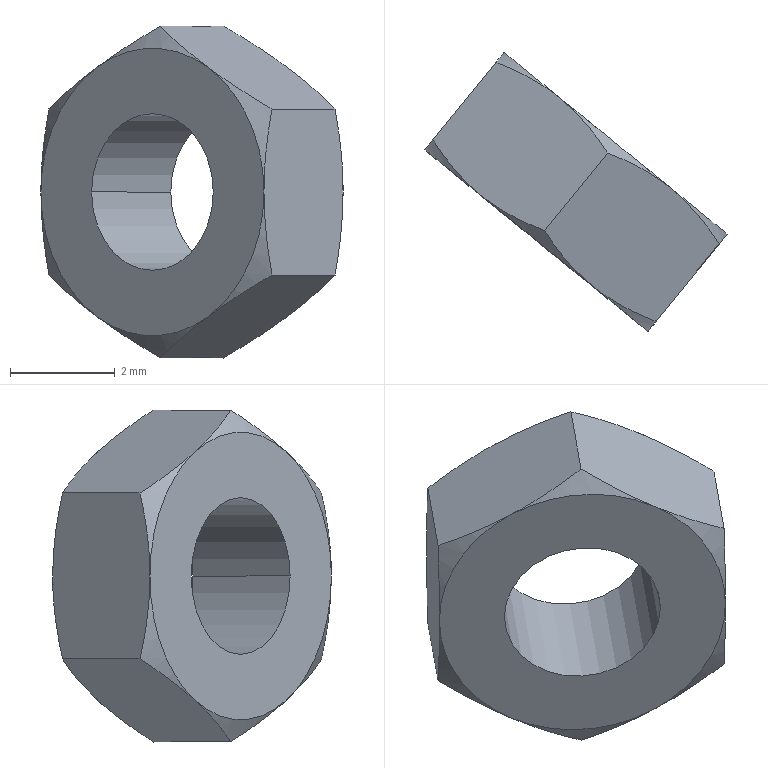Part | SolidWorks | features BaseBody 1 | 1 solid | 22 faces | box 5.781 x 5.332 x 6.351 mm | volume 45.543 mm3 | cone 12 | plane 8 | cylinder 2 | commonest cylinder face diameters 3 x2
STEP:
#1=CARTESIAN_POINT('',(505.624,-147.658,330.545));
#2=VERTEX_POINT('',#1);
#3=CARTESIAN_POINT('',(503.296,-145.766,330.545));
#4=VERTEX_POINT('',#3);
#5=CARTESIAN_POINT('',(504.46,-146.712,330.545));
#6=DIRECTION('',(0.6309,0.7758,-0.000000012));
#7=DIRECTION('',(-0.7758,0.6309,0.));
#8=AXIS2_PLACEMENT_3D('',#5,#6,#7);
#9=CIRCLE('',#8,1.5);
#10=EDGE_CURVE('',#2,#4,#9,.T.);
#11=ORIENTED_EDGE('',*,*,#10,.F.);
#12=CARTESIAN_POINT('',(507.138,-145.796,330.545));
#13=VERTEX_POINT('',#12);
#14=CARTESIAN_POINT('',(507.138,-145.796,330.545));
#15=DIRECTION('',(0.6309,0.7758,-0.000000012));
#16=VECTOR('',#15,1000.);
#17=LINE('',#14,#16);
#18=EDGE_CURVE('',#2,#13,#17,.T.);
#19=ORIENTED_EDGE('',*,*,#18,.T.);
#20=CARTESIAN_POINT('',(504.81,-143.904,330.545));
#21=VERTEX_POINT('',#20);
#22=CARTESIAN_POINT('',(505.974,-144.85,330.545));
#23=DIRECTION('',(0.6309,0.7758,-0.000000012));
#24=DIRECTION('',(-0.7758,0.6309,0.));
#25=AXIS2_PLACEMENT_3D('',#22,#23,#24);
#26=CIRCLE('',#25,1.5);
#27=EDGE_CURVE('',#13,#21,#26,.T.);
#28=ORIENTED_EDGE('',*,*,#27,.T.);
#29=CARTESIAN_POINT('',(504.81,-143.904,330.545));
#30=DIRECTION('',(0.6309,0.7758,-0.000000012));
#31=VECTOR('',#30,1000.);
#32=LINE('',#29,#31);
#33=EDGE_CURVE('',#4,#21,#32,.T.);
#34=ORIENTED_EDGE('',*,*,#33,.F.);
#35=EDGE_LOOP('',(#11,#19,#28,#34));
#36=FACE_OUTER_BOUND('',#35,.T.);
#37=CARTESIAN_POINT('',(505.974,-144.85,330.545));
#38=DIRECTION('',(0.6309,0.7758,-0.000000012));
#39=DIRECTION('',(-0.7758,0.6309,0.));
#40=AXIS2_PLACEMENT_3D('',#37,#38,#39);
#41=CYLINDRICAL_SURFACE('',#40,1.5);
#42=ADVANCED_FACE('',(#36),#41,.F.);
#43=CARTESIAN_POINT('',(505.974,-144.85,330.545));
#44=DIRECTION('',(0.6309,0.7758,-0.000000012));
#45=DIRECTION('',(-0.7758,0.6309,0.));
#46=AXIS2_PLACEMENT_3D('',#43,#44,#45);
#47=CIRCLE('',#46,1.5);
#48=EDGE_CURVE('',#21,#13,#47,.T.);
#49=ORIENTED_EDGE('',*,*,#48,.F.);
#50=ORIENTED_EDGE('',*,*,#27,.F.);
#51=EDGE_LOOP('',(#49,#50));
#52=FACE_BOUND('',#51,.T.);
#53=CARTESIAN_POINT('',(503.84,-143.115,330.545));
#54=VERTEX_POINT('',#53);
#55=CARTESIAN_POINT('',(504.907,-143.982,328.163));
#56=VERTEX_POINT('',#55);
#57=CARTESIAN_POINT('',(505.974,-144.85,330.545));
#58=DIRECTION('',(-0.6309,-0.7758,0.000000012));
#59=DIRECTION('',(0.7758,-0.6309,0.));
#60=AXIS2_PLACEMENT_3D('',#57,#58,#59);
#61=CIRCLE('',#60,2.75);
#62=EDGE_CURVE('',#54,#56,#61,.T.);
#63=ORIENTED_EDGE('',*,*,#62,.F.);
#64=CARTESIAN_POINT('',(504.907,-143.982,332.926));
#65=VERTEX_POINT('',#64);
#66=CARTESIAN_POINT('',(505.974,-144.85,330.545));
#67=DIRECTION('',(-0.6309,-0.7758,0.000000012));
#68=DIRECTION('',(0.7758,-0.6309,0.));
#69=AXIS2_PLACEMENT_3D('',#66,#67,#68);
#70=CIRCLE('',#69,2.75);
#71=EDGE_CURVE('',#65,#54,#70,.T.);
#72=ORIENTED_EDGE('',*,*,#71,.F.);
#73=CARTESIAN_POINT('',(507.041,-145.717,332.926));
#74=VERTEX_POINT('',#73);
#75=CARTESIAN_POINT('',(505.974,-144.85,330.545));
#76=DIRECTION('',(-0.6309,-0.7758,0.000000012));
#77=DIRECTION('',(0.7758,-0.6309,0.));
#78=AXIS2_PLACEMENT_3D('',#75,#76,#77);
#79=CIRCLE('',#78,2.75);
#80=EDGE_CURVE('',#74,#65,#79,.T.);
#81=ORIENTED_EDGE('',*,*,#80,.F.);
#82=CARTESIAN_POINT('',(508.108,-146.585,330.545));
#83=VERTEX_POINT('',#82);
#84=CARTESIAN_POINT('',(505.974,-144.85,330.545));
#85=DIRECTION('',(-0.6309,-0.7758,0.000000012));
#86=DIRECTION('',(0.7758,-0.6309,0.));
#87=AXIS2_PLACEMENT_3D('',#84,#85,#86);
#88=CIRCLE('',#87,2.75);
#89=EDGE_CURVE('',#83,#74,#88,.T.);
#90=ORIENTED_EDGE('',*,*,#89,.F.);
#91=CARTESIAN_POINT('',(507.041,-145.717,328.163));
#92=VERTEX_POINT('',#91);
#93=CARTESIAN_POINT('',(505.974,-144.85,330.545));
#94=DIRECTION('',(-0.6309,-0.7758,0.000000012));
#95=DIRECTION('',(0.7758,-0.6309,0.));
#96=AXIS2_PLACEMENT_3D('',#93,#94,#95);
#97=CIRCLE('',#96,2.75);
#98=EDGE_CURVE('',#92,#83,#97,.T.);
#99=ORIENTED_EDGE('',*,*,#98,.F.);
#100=CARTESIAN_POINT('',(505.974,-144.85,330.545));
#101=DIRECTION('',(-0.6309,-0.7758,0.000000012));
#102=DIRECTION('',(0.7758,-0.6309,0.));
#103=AXIS2_PLACEMENT_3D('',#100,#101,#102);
#104=CIRCLE('',#103,2.75);
#105=EDGE_CURVE('',#56,#92,#104,.T.);
#106=ORIENTED_EDGE('',*,*,#105,.F.);
#107=EDGE_LOOP('',(#63,#72,#81,#90,#99,#106));
#108=FACE_OUTER_BOUND('',#107,.T.);
#109=CARTESIAN_POINT('',(505.939,-144.821,330.545));
#110=DIRECTION('',(-0.6309,-0.7758,0.000000012));
#111=DIRECTION('',(0.7758,-0.6309,0.));
#112=AXIS2_PLACEMENT_3D('',#109,#110,#111);
#113=PLANE('',#112);
#114=ADVANCED_FACE('',(#52,#108),#113,.F.);
#115=ORIENTED_EDGE('',*,*,#18,.F.);
#116=CARTESIAN_POINT('',(504.46,-146.712,330.545));
#117=DIRECTION('',(0.6309,0.7758,-0.000000012));
#118=DIRECTION('',(-0.7758,0.6309,0.));
#119=AXIS2_PLACEMENT_3D('',#116,#117,#118);
#120=CIRCLE('',#119,1.5);
#121=EDGE_CURVE('',#4,#2,#120,.T.);
#122=ORIENTED_EDGE('',*,*,#121,.F.);
#123=ORIENTED_EDGE('',*,*,#33,.T.);
#124=ORIENTED_EDGE('',*,*,#48,.T.);
#125=EDGE_LOOP('',(#115,#122,#123,#124));
#126=FACE_OUTER_BOUND('',#125,.T.);
#127=CARTESIAN_POINT('',(505.974,-144.85,330.545));
#128=DIRECTION('',(0.6309,0.7758,-0.000000012));
#129=DIRECTION('',(-0.7758,0.6309,0.));
#130=AXIS2_PLACEMENT_3D('',#127,#128,#129);
#131=CYLINDRICAL_SURFACE('',#130,1.5);
#132=ADVANCED_FACE('',(#126),#131,.F.);
#133=ORIENTED_EDGE('',*,*,#105,.T.);
#134=CARTESIAN_POINT('',(505.819,-145.04,327.369));
#135=VERTEX_POINT('',#134);
#136=CARTESIAN_POINT('',(507.041,-145.717,328.163));
#137=CARTESIAN_POINT('',(506.677,-145.421,327.892));
#138=CARTESIAN_POINT('',(506.262,-145.208,327.628));
#139=CARTESIAN_POINT('',(505.819,-145.04,327.369));
#140=B_SPLINE_CURVE_WITH_KNOTS('',3,(#136,#137,#138,#139),.UNSPECIFIED.,.F.,.F.,(4,4),(0.,0.001607),.UNSPECIFIED.);
#141=EDGE_CURVE('',#92,#135,#140,.T.);
#142=ORIENTED_EDGE('',*,*,#141,.T.);
#143=CARTESIAN_POINT('',(504.907,-143.982,328.163));
#144=CARTESIAN_POINT('',(505.271,-144.278,327.892));
#145=CARTESIAN_POINT('',(505.565,-144.641,327.628));
#146=CARTESIAN_POINT('',(505.819,-145.04,327.369));
#147=B_SPLINE_CURVE_WITH_KNOTS('',3,(#143,#144,#145,#146),.UNSPECIFIED.,.F.,.F.,(4,4),(0.,0.001607),.UNSPECIFIED.);
#148=EDGE_CURVE('',#56,#135,#147,.T.);
#149=ORIENTED_EDGE('',*,*,#148,.F.);
#150=EDGE_LOOP('',(#133,#142,#149));
#151=FACE_OUTER_BOUND('',#150,.T.);
#152=CARTESIAN_POINT('',(505.818,-145.042,330.545));
#153=DIRECTION('',(-0.6309,-0.7758,0.000000012));
#154=DIRECTION('',(0.7758,-0.6309,0.));
#155=AXIS2_PLACEMENT_3D('',#152,#153,#154);
#156=CONICAL_SURFACE('',#155,3.178,1.047);
#157=ADVANCED_FACE('',(#151),#156,.T.);
#158=ORIENTED_EDGE('',*,*,#62,.T.);
#159=CARTESIAN_POINT('',(503.685,-143.305,328.957));
#160=VERTEX_POINT('',#159);
#161=CARTESIAN_POINT('',(503.685,-143.305,328.957));
#162=CARTESIAN_POINT('',(504.129,-143.473,328.697));
#163=CARTESIAN_POINT('',(504.543,-143.686,328.434));
#164=CARTESIAN_POINT('',(504.907,-143.982,328.163));
#165=B_SPLINE_CURVE_WITH_KNOTS('',3,(#161,#162,#163,#164),.UNSPECIFIED.,.F.,.F.,(4,4),(0.,0.001607),.UNSPECIFIED.);
#166=EDGE_CURVE('',#160,#56,#165,.T.);
#167=ORIENTED_EDGE('',*,*,#166,.F.);
#168=CARTESIAN_POINT('',(503.84,-143.115,330.545));
#169=CARTESIAN_POINT('',(503.84,-143.115,330.003));
#170=CARTESIAN_POINT('',(503.78,-143.189,329.476));
#171=CARTESIAN_POINT('',(503.685,-143.305,328.957));
#172=B_SPLINE_CURVE_WITH_KNOTS('',3,(#168,#169,#170,#171),.UNSPECIFIED.,.F.,.F.,(4,4),(0.,0.001607),.UNSPECIFIED.);
#173=EDGE_CURVE('',#54,#160,#172,.T.);
#174=ORIENTED_EDGE('',*,*,#173,.F.);
#175=EDGE_LOOP('',(#158,#167,#174));
#176=FACE_OUTER_BOUND('',#175,.T.);
#177=CARTESIAN_POINT('',(505.818,-145.042,330.545));
#178=DIRECTION('',(-0.6309,-0.7758,0.000000012));
#179=DIRECTION('',(0.7758,-0.6309,0.));
#180=AXIS2_PLACEMENT_3D('',#177,#178,#179);
#181=CONICAL_SURFACE('',#180,3.178,1.047);
#182=ADVANCED_FACE('',(#176),#181,.T.);
#183=ORIENTED_EDGE('',*,*,#71,.T.);
#184=CARTESIAN_POINT('',(503.685,-143.305,332.132));
#185=VERTEX_POINT('',#184);
#186=CARTESIAN_POINT('',(503.685,-143.305,332.132));
#187=CARTESIAN_POINT('',(503.78,-143.189,331.614));
#188=CARTESIAN_POINT('',(503.84,-143.115,331.086));
#189=CARTESIAN_POINT('',(503.84,-143.115,330.545));
#190=B_SPLINE_CURVE_WITH_KNOTS('',3,(#186,#187,#188,#189),.UNSPECIFIED.,.F.,.F.,(4,4),(0.,0.001607),.UNSPECIFIED.);
#191=EDGE_CURVE('',#185,#54,#190,.T.);
#192=ORIENTED_EDGE('',*,*,#191,.F.);
#193=CARTESIAN_POINT('',(504.907,-143.982,332.926));
#194=CARTESIAN_POINT('',(504.543,-143.686,332.655));
#195=CARTESIAN_POINT('',(504.129,-143.473,332.392));
#196=CARTESIAN_POINT('',(503.685,-143.305,332.132));
#197=B_SPLINE_CURVE_WITH_KNOTS('',3,(#193,#194,#195,#196),.UNSPECIFIED.,.F.,.F.,(4,4),(0.,0.001607),.UNSPECIFIED.);
#198=EDGE_CURVE('',#65,#185,#197,.T.);
#199=ORIENTED_EDGE('',*,*,#198,.F.);
#200=EDGE_LOOP('',(#183,#192,#199));
#201=FACE_OUTER_BOUND('',#200,.T.);
#202=CARTESIAN_POINT('',(505.818,-145.042,330.545));
#203=DIRECTION('',(-0.6309,-0.7758,0.000000012));
#204=DIRECTION('',(0.7758,-0.6309,0.));
#205=AXIS2_PLACEMENT_3D('',#202,#203,#204);
#206=CONICAL_SURFACE('',#205,3.178,1.047);
#207=ADVANCED_FACE('',(#201),#206,.T.);
#208=ORIENTED_EDGE('',*,*,#80,.T.);
#209=CARTESIAN_POINT('',(505.819,-145.04,333.72));
#210=VERTEX_POINT('',#209);
#211=CARTESIAN_POINT('',(505.819,-145.04,333.72));
#212=CARTESIAN_POINT('',(505.565,-144.641,333.461));
#213=CARTESIAN_POINT('',(505.271,-144.278,333.197));
#214=CARTESIAN_POINT('',(504.907,-143.982,332.926));
#215=B_SPLINE_CURVE_WITH_KNOTS('',3,(#211,#212,#213,#214),.UNSPECIFIED.,.F.,.F.,(4,4),(0.,0.001607),.UNSPECIFIED.);
#216=EDGE_CURVE('',#210,#65,#215,.T.);
#217=ORIENTED_EDGE('',*,*,#216,.F.);
#218=CARTESIAN_POINT('',(507.041,-145.717,332.926));
#219=CARTESIAN_POINT('',(506.677,-145.421,333.197));
#220=CARTESIAN_POINT('',(506.262,-145.208,333.461));
#221=CARTESIAN_POINT('',(505.819,-145.04,333.72));
#222=B_SPLINE_CURVE_WITH_KNOTS('',3,(#218,#219,#220,#221),.UNSPECIFIED.,.F.,.F.,(4,4),(0.,0.001607),.UNSPECIFIED.);
#223=EDGE_CURVE('',#74,#210,#222,.T.);
#224=ORIENTED_EDGE('',*,*,#223,.F.);
#225=EDGE_LOOP('',(#208,#217,#224));
#226=FACE_OUTER_BOUND('',#225,.T.);
#227=CARTESIAN_POINT('',(505.818,-145.042,330.545));
#228=DIRECTION('',(-0.6309,-0.7758,0.000000012));
#229=DIRECTION('',(0.7758,-0.6309,0.));
#230=AXIS2_PLACEMENT_3D('',#227,#228,#229);
#231=CONICAL_SURFACE('',#230,3.178,1.047);
#232=ADVANCED_FACE('',(#226),#231,.T.);
#233=CARTESIAN_POINT('',(507.953,-146.776,332.132));
#234=VERTEX_POINT('',#233);
#235=CARTESIAN_POINT('',(508.108,-146.585,330.545));
#236=CARTESIAN_POINT('',(508.108,-146.585,331.086));
#237=CARTESIAN_POINT('',(508.047,-146.659,331.614));
#238=CARTESIAN_POINT('',(507.953,-146.776,332.132));
#239=B_SPLINE_CURVE_WITH_KNOTS('',3,(#235,#236,#237,#238),.UNSPECIFIED.,.F.,.F.,(4,4),(0.,0.001607),.UNSPECIFIED.);
#240=EDGE_CURVE('',#83,#234,#239,.T.);
#241=ORIENTED_EDGE('',*,*,#240,.F.);
#242=ORIENTED_EDGE('',*,*,#89,.T.);
#243=CARTESIAN_POINT('',(507.953,-146.776,332.132));
#244=CARTESIAN_POINT('',(507.699,-146.376,332.392));
#245=CARTESIAN_POINT('',(507.405,-146.014,332.655));
#246=CARTESIAN_POINT('',(507.041,-145.717,332.926));
#247=B_SPLINE_CURVE_WITH_KNOTS('',3,(#243,#244,#245,#246),.UNSPECIFIED.,.F.,.F.,(4,4),(0.,0.001607),.UNSPECIFIED.);
#248=EDGE_CURVE('',#234,#74,#247,.T.);
#249=ORIENTED_EDGE('',*,*,#248,.F.);
#250=EDGE_LOOP('',(#241,#242,#249));
#251=FACE_OUTER_BOUND('',#250,.T.);
#252=CARTESIAN_POINT('',(505.818,-145.042,330.545));
#253=DIRECTION('',(-0.6309,-0.7758,0.000000012));
#254=DIRECTION('',(0.7758,-0.6309,0.));
#255=AXIS2_PLACEMENT_3D('',#252,#253,#254);
#256=CONICAL_SURFACE('',#255,3.178,1.047);
#257=ADVANCED_FACE('',(#251),#256,.T.);
#258=CARTESIAN_POINT('',(507.953,-146.776,328.957));
#259=VERTEX_POINT('',#258);
#260=CARTESIAN_POINT('',(507.953,-146.776,328.957));
#261=CARTESIAN_POINT('',(507.699,-146.376,328.697));
#262=CARTESIAN_POINT('',(507.405,-146.014,328.434));
#263=CARTESIAN_POINT('',(507.041,-145.717,328.163));
#264=B_SPLINE_CURVE_WITH_KNOTS('',3,(#260,#261,#262,#263),.UNSPECIFIED.,.F.,.F.,(4,4),(0.,0.001607),.UNSPECIFIED.);
#265=EDGE_CURVE('',#259,#92,#264,.T.);
#266=ORIENTED_EDGE('',*,*,#265,.T.);
#267=ORIENTED_EDGE('',*,*,#98,.T.);
#268=CARTESIAN_POINT('',(507.953,-146.776,328.957));
#269=CARTESIAN_POINT('',(508.047,-146.659,329.476));
#270=CARTESIAN_POINT('',(508.108,-146.585,330.003));
#271=CARTESIAN_POINT('',(508.108,-146.585,330.545));
#272=B_SPLINE_CURVE_WITH_KNOTS('',3,(#268,#269,#270,#271),.UNSPECIFIED.,.F.,.F.,(4,4),(0.,0.001607),.UNSPECIFIED.);
#273=EDGE_CURVE('',#259,#83,#272,.T.);
#274=ORIENTED_EDGE('',*,*,#273,.F.);
#275=EDGE_LOOP('',(#266,#267,#274));
#276=FACE_OUTER_BOUND('',#275,.T.);
#277=CARTESIAN_POINT('',(505.818,-145.042,330.545));
#278=DIRECTION('',(-0.6309,-0.7758,0.000000012));
#279=DIRECTION('',(0.7758,-0.6309,0.));
#280=AXIS2_PLACEMENT_3D('',#277,#278,#279);
#281=CONICAL_SURFACE('',#280,3.178,1.047);
#282=ADVANCED_FACE('',(#276),#281,.T.);
#283=ORIENTED_EDGE('',*,*,#121,.T.);
#284=ORIENTED_EDGE('',*,*,#10,.T.);
#285=EDGE_LOOP('',(#283,#284));
#286=FACE_BOUND('',#285,.T.);
#287=CARTESIAN_POINT('',(503.393,-145.844,328.163));
#288=VERTEX_POINT('',#287);
#289=CARTESIAN_POINT('',(505.527,-147.579,328.163));
#290=VERTEX_POINT('',#289);
#291=CARTESIAN_POINT('',(504.46,-146.712,330.545));
#292=DIRECTION('',(-0.6309,-0.7758,0.000000012));
#293=DIRECTION('',(-0.7758,0.6309,0.));
#294=AXIS2_PLACEMENT_3D('',#291,#292,#293);
#295=CIRCLE('',#294,2.75);
#296=EDGE_CURVE('',#288,#290,#295,.T.);
#297=ORIENTED_EDGE('',*,*,#296,.T.);
#298=CARTESIAN_POINT('',(506.593,-148.447,330.545));
#299=VERTEX_POINT('',#298);
#300=CARTESIAN_POINT('',(504.46,-146.712,330.545));
#301=DIRECTION('',(-0.6309,-0.7758,0.000000012));
#302=DIRECTION('',(-0.7758,0.6309,0.));
#303=AXIS2_PLACEMENT_3D('',#300,#301,#302);
#304=CIRCLE('',#303,2.75);
#305=EDGE_CURVE('',#290,#299,#304,.T.);
#306=ORIENTED_EDGE('',*,*,#305,.T.);
#307=CARTESIAN_POINT('',(505.527,-147.579,332.926));
#308=VERTEX_POINT('',#307);
#309=CARTESIAN_POINT('',(504.46,-146.712,330.545));
#310=DIRECTION('',(-0.6309,-0.7758,0.000000012));
#311=DIRECTION('',(-0.7758,0.6309,0.));
#312=AXIS2_PLACEMENT_3D('',#309,#310,#311);
#313=CIRCLE('',#312,2.75);
#314=EDGE_CURVE('',#299,#308,#313,.T.);
#315=ORIENTED_EDGE('',*,*,#314,.T.);
#316=CARTESIAN_POINT('',(503.393,-145.844,332.926));
#317=VERTEX_POINT('',#316);
#318=CARTESIAN_POINT('',(504.46,-146.712,330.545));
#319=DIRECTION('',(-0.6309,-0.7758,0.000000012));
#320=DIRECTION('',(-0.7758,0.6309,0.));
#321=AXIS2_PLACEMENT_3D('',#318,#319,#320);
#322=CIRCLE('',#321,2.75);
#323=EDGE_CURVE('',#308,#317,#322,.T.);
#324=ORIENTED_EDGE('',*,*,#323,.T.);
#325=CARTESIAN_POINT('',(502.326,-144.977,330.545));
#326=VERTEX_POINT('',#325);
#327=CARTESIAN_POINT('',(504.46,-146.712,330.545));
#328=DIRECTION('',(-0.6309,-0.7758,0.000000012));
#329=DIRECTION('',(-0.7758,0.6309,0.));
#330=AXIS2_PLACEMENT_3D('',#327,#328,#329);
#331=CIRCLE('',#330,2.75);
#332=EDGE_CURVE('',#317,#326,#331,.T.);
#333=ORIENTED_EDGE('',*,*,#332,.T.);
#334=CARTESIAN_POINT('',(504.46,-146.712,330.545));
#335=DIRECTION('',(-0.6309,-0.7758,0.000000012));
#336=DIRECTION('',(-0.7758,0.6309,0.));
#337=AXIS2_PLACEMENT_3D('',#334,#335,#336);
#338=CIRCLE('',#337,2.75);
#339=EDGE_CURVE('',#326,#288,#338,.T.);
#340=ORIENTED_EDGE('',*,*,#339,.T.);
#341=EDGE_LOOP('',(#297,#306,#315,#324,#333,#340));
#342=FACE_OUTER_BOUND('',#341,.T.);
#343=CARTESIAN_POINT('',(504.425,-146.683,330.545));
#344=DIRECTION('',(-0.6309,-0.7758,0.000000012));
#345=DIRECTION('',(0.7758,-0.6309,0.));
#346=AXIS2_PLACEMENT_3D('',#343,#344,#345);
#347=PLANE('',#346);
#348=ADVANCED_FACE('',(#286,#342),#347,.T.);
#349=CARTESIAN_POINT('',(506.748,-148.256,328.957));
#350=VERTEX_POINT('',#349);
#351=CARTESIAN_POINT('',(507.953,-146.776,328.957));
#352=DIRECTION('',(-0.6309,-0.7758,0.000000012));
#353=VECTOR('',#352,1000.);
#354=LINE('',#351,#353);
#355=EDGE_CURVE('',#259,#350,#354,.T.);
#356=ORIENTED_EDGE('',*,*,#355,.T.);
#357=CARTESIAN_POINT('',(506.748,-148.256,328.957));
#358=CARTESIAN_POINT('',(506.305,-148.089,328.697));
#359=CARTESIAN_POINT('',(505.891,-147.876,328.434));
#360=CARTESIAN_POINT('',(505.527,-147.579,328.163));
#361=B_SPLINE_CURVE_WITH_KNOTS('',3,(#357,#358,#359,#360),.UNSPECIFIED.,.F.,.F.,(4,4),(0.,0.001607),.UNSPECIFIED.);
#362=EDGE_CURVE('',#350,#290,#361,.T.);
#363=ORIENTED_EDGE('',*,*,#362,.T.);
#364=CARTESIAN_POINT('',(504.615,-146.521,327.369));
#365=VERTEX_POINT('',#364);
#366=CARTESIAN_POINT('',(505.527,-147.579,328.163));
#367=CARTESIAN_POINT('',(505.162,-147.283,327.892));
#368=CARTESIAN_POINT('',(504.869,-146.921,327.628));
#369=CARTESIAN_POINT('',(504.615,-146.521,327.369));
#370=B_SPLINE_CURVE_WITH_KNOTS('',3,(#366,#367,#368,#369),.UNSPECIFIED.,.F.,.F.,(4,4),(0.,0.001607),.UNSPECIFIED.);
#371=EDGE_CURVE('',#290,#365,#370,.T.);
#372=ORIENTED_EDGE('',*,*,#371,.T.);
#373=CARTESIAN_POINT('',(504.615,-146.521,327.369));
#374=DIRECTION('',(0.6309,0.7758,-0.000000012));
#375=VECTOR('',#374,1000.);
#376=LINE('',#373,#375);
#377=EDGE_CURVE('',#365,#135,#376,.T.);
#378=ORIENTED_EDGE('',*,*,#377,.T.);
#379=ORIENTED_EDGE('',*,*,#141,.F.);
#380=ORIENTED_EDGE('',*,*,#265,.F.);
#381=EDGE_LOOP('',(#356,#363,#372,#378,#379,#380));
#382=FACE_OUTER_BOUND('',#381,.T.);
#383=CARTESIAN_POINT('',(508.108,-146.585,328.957));
#384=DIRECTION('',(0.3879,-0.3155,-0.866));
#385=DIRECTION('',(-0.9126,0.,-0.4088));
#386=AXIS2_PLACEMENT_3D('',#383,#384,#385);
#387=PLANE('',#386);
#388=ADVANCED_FACE('',(#382),#387,.T.);
#389=CARTESIAN_POINT('',(506.748,-148.256,328.957));
#390=CARTESIAN_POINT('',(506.654,-148.373,329.476));
#391=CARTESIAN_POINT('',(506.593,-148.447,330.003));
#392=CARTESIAN_POINT('',(506.593,-148.447,330.545));
#393=B_SPLINE_CURVE_WITH_KNOTS('',3,(#389,#390,#391,#392),.UNSPECIFIED.,.F.,.F.,(4,4),(0.,0.001607),.UNSPECIFIED.);
#394=EDGE_CURVE('',#350,#299,#393,.T.);
#395=ORIENTED_EDGE('',*,*,#394,.T.);
#396=ORIENTED_EDGE('',*,*,#305,.F.);
#397=ORIENTED_EDGE('',*,*,#362,.F.);
#398=EDGE_LOOP('',(#395,#396,#397));
#399=FACE_OUTER_BOUND('',#398,.T.);
#400=CARTESIAN_POINT('',(504.616,-146.52,330.545));
#401=DIRECTION('',(0.6309,0.7758,-0.000000012));
#402=DIRECTION('',(-0.7758,0.6309,0.));
#403=AXIS2_PLACEMENT_3D('',#400,#401,#402);
#404=CONICAL_SURFACE('',#403,3.178,1.047);
#405=ADVANCED_FACE('',(#399),#404,.T.);
#406=ORIENTED_EDGE('',*,*,#371,.F.);
#407=ORIENTED_EDGE('',*,*,#296,.F.);
#408=CARTESIAN_POINT('',(503.393,-145.844,328.163));
#409=CARTESIAN_POINT('',(503.757,-146.14,327.892));
#410=CARTESIAN_POINT('',(504.172,-146.354,327.628));
#411=CARTESIAN_POINT('',(504.615,-146.521,327.369));
#412=B_SPLINE_CURVE_WITH_KNOTS('',3,(#408,#409,#410,#411),.UNSPECIFIED.,.F.,.F.,(4,4),(0.,0.001607),.UNSPECIFIED.);
#413=EDGE_CURVE('',#288,#365,#412,.T.);
#414=ORIENTED_EDGE('',*,*,#413,.T.);
#415=EDGE_LOOP('',(#406,#407,#414));
#416=FACE_OUTER_BOUND('',#415,.T.);
#417=CARTESIAN_POINT('',(504.616,-146.52,330.545));
#418=DIRECTION('',(0.6309,0.7758,-0.000000012));
#419=DIRECTION('',(-0.7758,0.6309,0.));
#420=AXIS2_PLACEMENT_3D('',#417,#418,#419);
#421=CONICAL_SURFACE('',#420,3.178,1.047);
#422=ADVANCED_FACE('',(#416),#421,.T.);
#423=CARTESIAN_POINT('',(502.481,-144.786,328.957));
#424=VERTEX_POINT('',#423);
#425=CARTESIAN_POINT('',(502.481,-144.786,328.957));
#426=CARTESIAN_POINT('',(502.735,-145.186,328.697));
#427=CARTESIAN_POINT('',(503.029,-145.548,328.434));
#428=CARTESIAN_POINT('',(503.393,-145.844,328.163));
#429=B_SPLINE_CURVE_WITH_KNOTS('',3,(#425,#426,#427,#428),.UNSPECIFIED.,.F.,.F.,(4,4),(0.,0.001607),.UNSPECIFIED.);
#430=EDGE_CURVE('',#424,#288,#429,.T.);
#431=ORIENTED_EDGE('',*,*,#430,.T.);
#432=ORIENTED_EDGE('',*,*,#339,.F.);
#433=CARTESIAN_POINT('',(502.481,-144.786,328.957));
#434=CARTESIAN_POINT('',(502.387,-144.902,329.476));
#435=CARTESIAN_POINT('',(502.326,-144.977,330.003));
#436=CARTESIAN_POINT('',(502.326,-144.977,330.545));
#437=B_SPLINE_CURVE_WITH_KNOTS('',3,(#433,#434,#435,#436),.UNSPECIFIED.,.F.,.F.,(4,4),(0.,0.001607),.UNSPECIFIED.);
#438=EDGE_CURVE('',#424,#326,#437,.T.);
#439=ORIENTED_EDGE('',*,*,#438,.F.);
#440=EDGE_LOOP('',(#431,#432,#439));
#441=FACE_OUTER_BOUND('',#440,.T.);
#442=CARTESIAN_POINT('',(504.616,-146.52,330.545));
#443=DIRECTION('',(0.6309,0.7758,-0.000000012));
#444=DIRECTION('',(-0.7758,0.6309,0.));
#445=AXIS2_PLACEMENT_3D('',#442,#443,#444);
#446=CONICAL_SURFACE('',#445,3.178,1.047);
#447=ADVANCED_FACE('',(#441),#446,.T.);
#448=ORIENTED_EDGE('',*,*,#332,.F.);
#449=CARTESIAN_POINT('',(502.481,-144.786,332.132));
#450=VERTEX_POINT('',#449);
#451=CARTESIAN_POINT('',(502.481,-144.786,332.132));
#452=CARTESIAN_POINT('',(502.735,-145.186,332.392));
#453=CARTESIAN_POINT('',(503.029,-145.548,332.655));
#454=CARTESIAN_POINT('',(503.393,-145.844,332.926));
#455=B_SPLINE_CURVE_WITH_KNOTS('',3,(#451,#452,#453,#454),.UNSPECIFIED.,.F.,.F.,(4,4),(0.,0.001607),.UNSPECIFIED.);
#456=EDGE_CURVE('',#450,#317,#455,.T.);
#457=ORIENTED_EDGE('',*,*,#456,.F.);
#458=CARTESIAN_POINT('',(502.326,-144.977,330.545));
#459=CARTESIAN_POINT('',(502.326,-144.977,331.086));
#460=CARTESIAN_POINT('',(502.387,-144.902,331.614));
#461=CARTESIAN_POINT('',(502.481,-144.786,332.132));
#462=B_SPLINE_CURVE_WITH_KNOTS('',3,(#458,#459,#460,#461),.UNSPECIFIED.,.F.,.F.,(4,4),(0.,0.001607),.UNSPECIFIED.);
#463=EDGE_CURVE('',#326,#450,#462,.T.);
#464=ORIENTED_EDGE('',*,*,#463,.F.);
#465=EDGE_LOOP('',(#448,#457,#464));
#466=FACE_OUTER_BOUND('',#465,.T.);
#467=CARTESIAN_POINT('',(504.616,-146.52,330.545));
#468=DIRECTION('',(0.6309,0.7758,-0.000000012));
#469=DIRECTION('',(-0.7758,0.6309,0.));
#470=AXIS2_PLACEMENT_3D('',#467,#468,#469);
#471=CONICAL_SURFACE('',#470,3.178,1.047);
#472=ADVANCED_FACE('',(#466),#471,.T.);
#473=ORIENTED_EDGE('',*,*,#323,.F.);
#474=CARTESIAN_POINT('',(504.615,-146.521,333.72));
#475=VERTEX_POINT('',#474);
#476=CARTESIAN_POINT('',(504.615,-146.521,333.72));
#477=CARTESIAN_POINT('',(504.869,-146.921,333.461));
#478=CARTESIAN_POINT('',(505.162,-147.283,333.197));
#479=CARTESIAN_POINT('',(505.527,-147.579,332.926));
#480=B_SPLINE_CURVE_WITH_KNOTS('',3,(#476,#477,#478,#479),.UNSPECIFIED.,.F.,.F.,(4,4),(0.,0.001607),.UNSPECIFIED.);
#481=EDGE_CURVE('',#475,#308,#480,.T.);
#482=ORIENTED_EDGE('',*,*,#481,.F.);
#483=CARTESIAN_POINT('',(503.393,-145.844,332.926));
#484=CARTESIAN_POINT('',(503.757,-146.14,333.197));
#485=CARTESIAN_POINT('',(504.172,-146.354,333.461));
#486=CARTESIAN_POINT('',(504.615,-146.521,333.72));
#487=B_SPLINE_CURVE_WITH_KNOTS('',3,(#483,#484,#485,#486),.UNSPECIFIED.,.F.,.F.,(4,4),(0.,0.001607),.UNSPECIFIED.);
#488=EDGE_CURVE('',#317,#475,#487,.T.);
#489=ORIENTED_EDGE('',*,*,#488,.F.);
#490=EDGE_LOOP('',(#473,#482,#489));
#491=FACE_OUTER_BOUND('',#490,.T.);
#492=CARTESIAN_POINT('',(504.616,-146.52,330.545));
#493=DIRECTION('',(0.6309,0.7758,-0.000000012));
#494=DIRECTION('',(-0.7758,0.6309,0.));
#495=AXIS2_PLACEMENT_3D('',#492,#493,#494);
#496=CONICAL_SURFACE('',#495,3.178,1.047);
#497=ADVANCED_FACE('',(#491),#496,.T.);
#498=ORIENTED_EDGE('',*,*,#314,.F.);
#499=CARTESIAN_POINT('',(506.748,-148.256,332.132));
#500=VERTEX_POINT('',#499);
#501=CARTESIAN_POINT('',(506.593,-148.447,330.545));
#502=CARTESIAN_POINT('',(506.593,-148.447,331.086));
#503=CARTESIAN_POINT('',(506.654,-148.373,331.614));
#504=CARTESIAN_POINT('',(506.748,-148.256,332.132));
#505=B_SPLINE_CURVE_WITH_KNOTS('',3,(#501,#502,#503,#504),.UNSPECIFIED.,.F.,.F.,(4,4),(0.,0.001607),.UNSPECIFIED.);
#506=EDGE_CURVE('',#299,#500,#505,.T.);
#507=ORIENTED_EDGE('',*,*,#506,.T.);
#508=CARTESIAN_POINT('',(505.527,-147.579,332.926));
#509=CARTESIAN_POINT('',(505.891,-147.876,332.655));
#510=CARTESIAN_POINT('',(506.305,-148.089,332.392));
#511=CARTESIAN_POINT('',(506.748,-148.256,332.132));
#512=B_SPLINE_CURVE_WITH_KNOTS('',3,(#508,#509,#510,#511),.UNSPECIFIED.,.F.,.F.,(4,4),(0.,0.001607),.UNSPECIFIED.);
#513=EDGE_CURVE('',#308,#500,#512,.T.);
#514=ORIENTED_EDGE('',*,*,#513,.F.);
#515=EDGE_LOOP('',(#498,#507,#514));
#516=FACE_OUTER_BOUND('',#515,.T.);
#517=CARTESIAN_POINT('',(504.616,-146.52,330.545));
#518=DIRECTION('',(0.6309,0.7758,-0.000000012));
#519=DIRECTION('',(-0.7758,0.6309,0.));
#520=AXIS2_PLACEMENT_3D('',#517,#518,#519);
#521=CONICAL_SURFACE('',#520,3.178,1.047);
#522=ADVANCED_FACE('',(#516),#521,.T.);
#523=CARTESIAN_POINT('',(508.108,-146.585,332.132));
#524=DIRECTION('',(-0.6309,-0.7758,0.));
#525=VECTOR('',#524,1000.);
#526=LINE('',#523,#525);
#527=EDGE_CURVE('',#234,#500,#526,.T.);
#528=ORIENTED_EDGE('',*,*,#527,.T.);
#529=ORIENTED_EDGE('',*,*,#506,.F.);
#530=ORIENTED_EDGE('',*,*,#394,.F.);
#531=ORIENTED_EDGE('',*,*,#355,.F.);
#532=ORIENTED_EDGE('',*,*,#273,.T.);
#533=ORIENTED_EDGE('',*,*,#240,.T.);
#534=EDGE_LOOP('',(#528,#529,#530,#531,#532,#533));
#535=FACE_OUTER_BOUND('',#534,.T.);
#536=CARTESIAN_POINT('',(508.108,-146.585,332.132));
#537=DIRECTION('',(0.7758,-0.6309,-0.000000021));
#538=DIRECTION('',(0.6309,0.7758,0.));
#539=AXIS2_PLACEMENT_3D('',#536,#537,#538);
#540=PLANE('',#539);
#541=ADVANCED_FACE('',(#535),#540,.T.);
#542=ORIENTED_EDGE('',*,*,#377,.F.);
#543=ORIENTED_EDGE('',*,*,#413,.F.);
#544=ORIENTED_EDGE('',*,*,#430,.F.);
#545=CARTESIAN_POINT('',(502.481,-144.786,328.957));
#546=DIRECTION('',(0.6309,0.7758,-0.000000012));
#547=VECTOR('',#546,1000.);
#548=LINE('',#545,#547);
#549=EDGE_CURVE('',#424,#160,#548,.T.);
#550=ORIENTED_EDGE('',*,*,#549,.T.);
#551=ORIENTED_EDGE('',*,*,#166,.T.);
#552=ORIENTED_EDGE('',*,*,#148,.T.);
#553=EDGE_LOOP('',(#542,#543,#544,#550,#551,#552));
#554=FACE_OUTER_BOUND('',#553,.T.);
#555=CARTESIAN_POINT('',(505.974,-144.85,327.369));
#556=DIRECTION('',(-0.3879,0.3155,-0.866));
#557=DIRECTION('',(-0.9126,0.,0.4088));
#558=AXIS2_PLACEMENT_3D('',#555,#556,#557);
#559=PLANE('',#558);
#560=ADVANCED_FACE('',(#554),#559,.T.);
#561=ORIENTED_EDGE('',*,*,#223,.T.);
#562=CARTESIAN_POINT('',(505.819,-145.04,333.72));
#563=DIRECTION('',(-0.6309,-0.7758,0.000000012));
#564=VECTOR('',#563,1000.);
#565=LINE('',#562,#564);
#566=EDGE_CURVE('',#210,#475,#565,.T.);
#567=ORIENTED_EDGE('',*,*,#566,.T.);
#568=ORIENTED_EDGE('',*,*,#481,.T.);
#569=ORIENTED_EDGE('',*,*,#513,.T.);
#570=ORIENTED_EDGE('',*,*,#527,.F.);
#571=ORIENTED_EDGE('',*,*,#248,.T.);
#572=EDGE_LOOP('',(#561,#567,#568,#569,#570,#571));
#573=FACE_OUTER_BOUND('',#572,.T.);
#574=CARTESIAN_POINT('',(505.974,-144.85,333.72));
#575=DIRECTION('',(0.3879,-0.3155,0.866));
#576=DIRECTION('',(0.9126,0.,-0.4088));
#577=AXIS2_PLACEMENT_3D('',#574,#575,#576);
#578=PLANE('',#577);
#579=ADVANCED_FACE('',(#573),#578,.T.);
#580=ORIENTED_EDGE('',*,*,#173,.T.);
#581=ORIENTED_EDGE('',*,*,#549,.F.);
#582=ORIENTED_EDGE('',*,*,#438,.T.);
#583=ORIENTED_EDGE('',*,*,#463,.T.);
#584=CARTESIAN_POINT('',(503.84,-143.115,332.132));
#585=DIRECTION('',(0.6309,0.7758,0.));
#586=VECTOR('',#585,1000.);
#587=LINE('',#584,#586);
#588=EDGE_CURVE('',#450,#185,#587,.T.);
#589=ORIENTED_EDGE('',*,*,#588,.T.);
#590=ORIENTED_EDGE('',*,*,#191,.T.);
#591=EDGE_LOOP('',(#580,#581,#582,#583,#589,#590));
#592=FACE_OUTER_BOUND('',#591,.T.);
#593=CARTESIAN_POINT('',(503.84,-143.115,328.957));
#594=DIRECTION('',(-0.7758,0.6309,0.000000021));
#595=DIRECTION('',(-0.6309,-0.7758,0.));
#596=AXIS2_PLACEMENT_3D('',#593,#594,#595);
#597=PLANE('',#596);
#598=ADVANCED_FACE('',(#592),#597,.T.);
#599=ORIENTED_EDGE('',*,*,#198,.T.);
#600=ORIENTED_EDGE('',*,*,#588,.F.);
#601=ORIENTED_EDGE('',*,*,#456,.T.);
#602=ORIENTED_EDGE('',*,*,#488,.T.);
#603=ORIENTED_EDGE('',*,*,#566,.F.);
#604=ORIENTED_EDGE('',*,*,#216,.T.);
#605=EDGE_LOOP('',(#599,#600,#601,#602,#603,#604));
#606=FACE_OUTER_BOUND('',#605,.T.);
#607=CARTESIAN_POINT('',(503.84,-143.115,332.132));
#608=DIRECTION('',(-0.3879,0.3155,0.866));
#609=DIRECTION('',(0.9126,0.,0.4088));
#610=AXIS2_PLACEMENT_3D('',#607,#608,#609);
#611=PLANE('',#610);
#612=ADVANCED_FACE('',(#606),#611,.T.);
#613=CLOSED_SHELL('',(#42,#114,#132,#157,#182,#207,#232,#257,#282,#348,#388,#405,#422,#447,#472,#497,#522,#541,#560,#579,#598,#612));
#614=MANIFOLD_SOLID_BREP('',#613);
#615=CARTESIAN_POINT('',(0.,0.,0.));
#616=DIRECTION('',(0.,0.,1.));
#617=DIRECTION('',(1.,0.,0.));
#618=AXIS2_PLACEMENT_3D('',#615,#616,#617);
#619=(LENGTH_UNIT()NAMED_UNIT(*)SI_UNIT(.MILLI.,.METRE.));
#620=UNCERTAINTY_MEASURE_WITH_UNIT(LENGTH_MEASURE(0.00001),#619,'','');
#621=(NAMED_UNIT(*)PLANE_ANGLE_UNIT()SI_UNIT($,.RADIAN.));
#622=(NAMED_UNIT(*)SI_UNIT($,.STERADIAN.)SOLID_ANGLE_UNIT());
#623=(GEOMETRIC_REPRESENTATION_CONTEXT(3)GLOBAL_UNCERTAINTY_ASSIGNED_CONTEXT((#620))GLOBAL_UNIT_ASSIGNED_CONTEXT((#619,#621,#622))REPRESENTATION_CONTEXT('',''));
#624=ADVANCED_BREP_SHAPE_REPRESENTATION('',(#614,#618),#623);